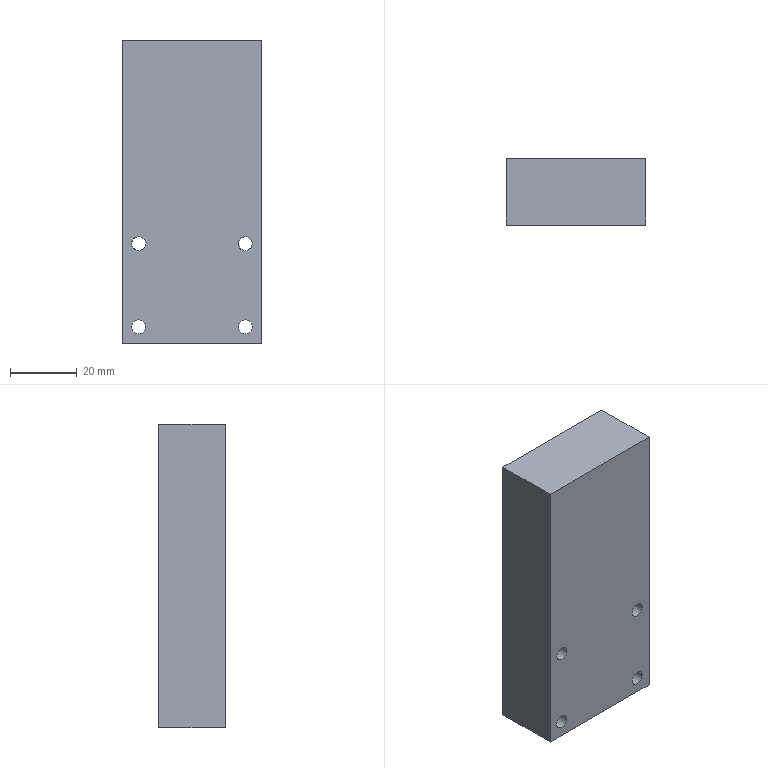Part | NX | features M5 螺纹孔1 2 | 1 solid | 10 faces | box 42 x 20 x 91 mm | volume 75332 mm3 | plane 6 | cylinder 4 | commonest cylinder face diameters 4.2 x4
STEP:
#1=CARTESIAN_POINT('',(16.,135.3,53.4));
#2=VERTEX_POINT('',#1);
#3=CARTESIAN_POINT('',(16.,135.3,55.5));
#4=DIRECTION('',(0.,-1.,0.));
#5=DIRECTION('',(0.,0.,-1.));
#6=AXIS2_PLACEMENT_3D('',#3,#4,#5);
#7=CIRCLE('',#6,2.1);
#8=EDGE_CURVE('',#2,#2,#7,.T.);
#9=ORIENTED_EDGE('',*,*,#8,.T.);
#10=EDGE_LOOP('',(#9));
#11=FACE_BOUND('',#10,.T.);
#12=CARTESIAN_POINT('',(16.,155.3,53.4));
#13=VERTEX_POINT('',#12);
#14=CARTESIAN_POINT('',(16.,155.3,55.5));
#15=DIRECTION('',(0.,-1.,0.));
#16=DIRECTION('',(0.,0.,-1.));
#17=AXIS2_PLACEMENT_3D('',#14,#15,#16);
#18=CIRCLE('',#17,2.1);
#19=EDGE_CURVE('',#13,#13,#18,.T.);
#20=ORIENTED_EDGE('',*,*,#19,.F.);
#21=EDGE_LOOP('',(#20));
#22=FACE_BOUND('',#21,.T.);
#23=CARTESIAN_POINT('',(16.,135.3,55.5));
#24=DIRECTION('',(0.,-1.,0.));
#25=DIRECTION('',(1.,0.,-0.000000009));
#26=AXIS2_PLACEMENT_3D('',#23,#24,#25);
#27=CYLINDRICAL_SURFACE('',#26,2.1);
#28=ADVANCED_FACE('',(#11,#22),#27,.F.);
#29=CARTESIAN_POINT('',(-16.,135.3,53.4));
#30=VERTEX_POINT('',#29);
#31=CARTESIAN_POINT('',(-16.,135.3,55.5));
#32=DIRECTION('',(0.,-1.,0.));
#33=DIRECTION('',(0.,0.,-1.));
#34=AXIS2_PLACEMENT_3D('',#31,#32,#33);
#35=CIRCLE('',#34,2.1);
#36=EDGE_CURVE('',#30,#30,#35,.T.);
#37=ORIENTED_EDGE('',*,*,#36,.T.);
#38=EDGE_LOOP('',(#37));
#39=FACE_BOUND('',#38,.T.);
#40=CARTESIAN_POINT('',(-16.,155.3,53.4));
#41=VERTEX_POINT('',#40);
#42=CARTESIAN_POINT('',(-16.,155.3,55.5));
#43=DIRECTION('',(0.,-1.,0.));
#44=DIRECTION('',(0.,0.,-1.));
#45=AXIS2_PLACEMENT_3D('',#42,#43,#44);
#46=CIRCLE('',#45,2.1);
#47=EDGE_CURVE('',#41,#41,#46,.T.);
#48=ORIENTED_EDGE('',*,*,#47,.F.);
#49=EDGE_LOOP('',(#48));
#50=FACE_BOUND('',#49,.T.);
#51=CARTESIAN_POINT('',(-16.,135.3,55.5));
#52=DIRECTION('',(0.,-1.,0.));
#53=DIRECTION('',(1.,0.,-0.000000009));
#54=AXIS2_PLACEMENT_3D('',#51,#52,#53);
#55=CYLINDRICAL_SURFACE('',#54,2.1);
#56=ADVANCED_FACE('',(#39,#50),#55,.F.);
#57=CARTESIAN_POINT('',(-21.,155.3,141.5));
#58=VERTEX_POINT('',#57);
#59=CARTESIAN_POINT('',(-21.,155.3,50.5));
#60=VERTEX_POINT('',#59);
#61=CARTESIAN_POINT('',(-21.,155.3,85.5));
#62=DIRECTION('',(-0.000000009,0.,-1.));
#63=VECTOR('',#62,1000.);
#64=LINE('',#61,#63);
#65=EDGE_CURVE('',#58,#60,#64,.T.);
#66=ORIENTED_EDGE('',*,*,#65,.T.);
#67=CARTESIAN_POINT('',(-21.,135.3,50.5));
#68=VERTEX_POINT('',#67);
#69=CARTESIAN_POINT('',(-21.,135.3,50.5));
#70=DIRECTION('',(0.,-1.,0.));
#71=VECTOR('',#70,1000.);
#72=LINE('',#69,#71);
#73=EDGE_CURVE('',#60,#68,#72,.T.);
#74=ORIENTED_EDGE('',*,*,#73,.T.);
#75=CARTESIAN_POINT('',(-21.,135.3,141.5));
#76=VERTEX_POINT('',#75);
#77=CARTESIAN_POINT('',(-21.,135.3,85.5));
#78=DIRECTION('',(0.000000009,0.,1.));
#79=VECTOR('',#78,1000.);
#80=LINE('',#77,#79);
#81=EDGE_CURVE('',#76,#68,#80,.F.);
#82=ORIENTED_EDGE('',*,*,#81,.F.);
#83=CARTESIAN_POINT('',(-21.,160.6,141.5));
#84=DIRECTION('',(0.,-1.,0.));
#85=VECTOR('',#84,1000.);
#86=LINE('',#83,#85);
#87=EDGE_CURVE('',#58,#76,#86,.T.);
#88=ORIENTED_EDGE('',*,*,#87,.F.);
#89=EDGE_LOOP('',(#66,#74,#82,#88));
#90=FACE_BOUND('',#89,.T.);
#91=CARTESIAN_POINT('',(-21.,135.3,85.5));
#92=DIRECTION('',(1.,0.,-0.000000009));
#93=DIRECTION('',(0.000000009,0.,1.));
#94=AXIS2_PLACEMENT_3D('',#91,#92,#93);
#95=PLANE('',#94);
#96=ADVANCED_FACE('',(#90),#95,.F.);
#97=CARTESIAN_POINT('',(21.,155.3,50.5));
#98=VERTEX_POINT('',#97);
#99=CARTESIAN_POINT('',(-25.,155.3,50.5));
#100=DIRECTION('',(1.,0.,-0.000000009));
#101=VECTOR('',#100,1000.);
#102=LINE('',#99,#101);
#103=EDGE_CURVE('',#60,#98,#102,.T.);
#104=ORIENTED_EDGE('',*,*,#103,.T.);
#105=CARTESIAN_POINT('',(21.,135.3,50.5));
#106=VERTEX_POINT('',#105);
#107=CARTESIAN_POINT('',(21.,89.3,50.5));
#108=DIRECTION('',(0.,-1.,0.));
#109=VECTOR('',#108,1000.);
#110=LINE('',#107,#109);
#111=EDGE_CURVE('',#98,#106,#110,.T.);
#112=ORIENTED_EDGE('',*,*,#111,.T.);
#113=CARTESIAN_POINT('',(-25.,135.3,50.5));
#114=DIRECTION('',(1.,0.,-0.000000009));
#115=VECTOR('',#114,1000.);
#116=LINE('',#113,#115);
#117=EDGE_CURVE('',#68,#106,#116,.T.);
#118=ORIENTED_EDGE('',*,*,#117,.F.);
#119=ORIENTED_EDGE('',*,*,#73,.F.);
#120=EDGE_LOOP('',(#104,#112,#118,#119));
#121=FACE_BOUND('',#120,.T.);
#122=CARTESIAN_POINT('',(-25.,89.3,50.5));
#123=DIRECTION('',(0.000000009,0.,1.));
#124=DIRECTION('',(0.,1.,0.));
#125=AXIS2_PLACEMENT_3D('',#122,#123,#124);
#126=PLANE('',#125);
#127=ADVANCED_FACE('',(#121),#126,.F.);
#128=CARTESIAN_POINT('',(21.,155.3,141.5));
#129=VERTEX_POINT('',#128);
#130=CARTESIAN_POINT('',(21.,155.3,85.5));
#131=DIRECTION('',(0.000000009,0.,1.));
#132=VECTOR('',#131,1000.);
#133=LINE('',#130,#132);
#134=EDGE_CURVE('',#98,#129,#133,.T.);
#135=ORIENTED_EDGE('',*,*,#134,.T.);
#136=CARTESIAN_POINT('',(21.,135.3,141.5));
#137=VERTEX_POINT('',#136);
#138=CARTESIAN_POINT('',(21.,135.3,141.5));
#139=DIRECTION('',(0.,-1.,0.));
#140=VECTOR('',#139,1000.);
#141=LINE('',#138,#140);
#142=EDGE_CURVE('',#129,#137,#141,.T.);
#143=ORIENTED_EDGE('',*,*,#142,.T.);
#144=CARTESIAN_POINT('',(21.,135.3,85.5));
#145=DIRECTION('',(-0.000000009,0.,-1.));
#146=VECTOR('',#145,1000.);
#147=LINE('',#144,#146);
#148=EDGE_CURVE('',#106,#137,#147,.F.);
#149=ORIENTED_EDGE('',*,*,#148,.F.);
#150=ORIENTED_EDGE('',*,*,#111,.F.);
#151=EDGE_LOOP('',(#135,#143,#149,#150));
#152=FACE_BOUND('',#151,.T.);
#153=CARTESIAN_POINT('',(21.,135.3,85.5));
#154=DIRECTION('',(-1.,0.,0.000000009));
#155=DIRECTION('',(-0.000000009,0.,-1.));
#156=AXIS2_PLACEMENT_3D('',#153,#154,#155);
#157=PLANE('',#156);
#158=ADVANCED_FACE('',(#152),#157,.F.);
#159=CARTESIAN_POINT('',(58.,155.3,141.5));
#160=DIRECTION('',(-1.,0.,0.000000019));
#161=VECTOR('',#160,1000.);
#162=LINE('',#159,#161);
#163=EDGE_CURVE('',#129,#58,#162,.T.);
#164=ORIENTED_EDGE('',*,*,#163,.T.);
#165=ORIENTED_EDGE('',*,*,#87,.T.);
#166=CARTESIAN_POINT('',(58.,135.3,141.5));
#167=DIRECTION('',(-1.,0.,0.000000019));
#168=VECTOR('',#167,1000.);
#169=LINE('',#166,#168);
#170=EDGE_CURVE('',#137,#76,#169,.T.);
#171=ORIENTED_EDGE('',*,*,#170,.F.);
#172=ORIENTED_EDGE('',*,*,#142,.F.);
#173=EDGE_LOOP('',(#164,#165,#171,#172));
#174=FACE_BOUND('',#173,.T.);
#175=CARTESIAN_POINT('',(58.,160.6,141.5));
#176=DIRECTION('',(-0.000000019,0.,-1.));
#177=DIRECTION('',(1.,0.,-0.000000019));
#178=AXIS2_PLACEMENT_3D('',#175,#176,#177);
#179=PLANE('',#178);
#180=ADVANCED_FACE('',(#174),#179,.F.);
#181=CARTESIAN_POINT('',(13.9,135.3,80.5));
#182=VERTEX_POINT('',#181);
#183=CARTESIAN_POINT('',(16.,135.3,80.5));
#184=DIRECTION('',(0.,1.,0.));
#185=DIRECTION('',(-1.,0.,0.000000009));
#186=AXIS2_PLACEMENT_3D('',#183,#184,#185);
#187=CIRCLE('',#186,2.1);
#188=EDGE_CURVE('',#182,#182,#187,.F.);
#189=ORIENTED_EDGE('',*,*,#188,.T.);
#190=EDGE_LOOP('',(#189));
#191=FACE_BOUND('',#190,.T.);
#192=CARTESIAN_POINT('',(16.,155.3,78.4));
#193=VERTEX_POINT('',#192);
#194=CARTESIAN_POINT('',(16.,155.3,80.5));
#195=DIRECTION('',(0.,-1.,0.));
#196=DIRECTION('',(0.,0.,-1.));
#197=AXIS2_PLACEMENT_3D('',#194,#195,#196);
#198=CIRCLE('',#197,2.1);
#199=EDGE_CURVE('',#193,#193,#198,.T.);
#200=ORIENTED_EDGE('',*,*,#199,.F.);
#201=EDGE_LOOP('',(#200));
#202=FACE_BOUND('',#201,.T.);
#203=CARTESIAN_POINT('',(16.,135.3,80.5));
#204=DIRECTION('',(0.,-1.,0.));
#205=DIRECTION('',(1.,0.,-0.000000009));
#206=AXIS2_PLACEMENT_3D('',#203,#204,#205);
#207=CYLINDRICAL_SURFACE('',#206,2.1);
#208=ADVANCED_FACE('',(#191,#202),#207,.F.);
#209=CARTESIAN_POINT('',(-18.1,135.3,80.5));
#210=VERTEX_POINT('',#209);
#211=CARTESIAN_POINT('',(-16.,135.3,80.5));
#212=DIRECTION('',(0.,1.,0.));
#213=DIRECTION('',(-1.,0.,0.000000009));
#214=AXIS2_PLACEMENT_3D('',#211,#212,#213);
#215=CIRCLE('',#214,2.1);
#216=EDGE_CURVE('',#210,#210,#215,.F.);
#217=ORIENTED_EDGE('',*,*,#216,.T.);
#218=EDGE_LOOP('',(#217));
#219=FACE_BOUND('',#218,.T.);
#220=CARTESIAN_POINT('',(-16.,155.3,78.4));
#221=VERTEX_POINT('',#220);
#222=CARTESIAN_POINT('',(-16.,155.3,80.5));
#223=DIRECTION('',(0.,-1.,0.));
#224=DIRECTION('',(0.,0.,-1.));
#225=AXIS2_PLACEMENT_3D('',#222,#223,#224);
#226=CIRCLE('',#225,2.1);
#227=EDGE_CURVE('',#221,#221,#226,.T.);
#228=ORIENTED_EDGE('',*,*,#227,.F.);
#229=EDGE_LOOP('',(#228));
#230=FACE_BOUND('',#229,.T.);
#231=CARTESIAN_POINT('',(-16.,135.3,80.5));
#232=DIRECTION('',(0.,-1.,0.));
#233=DIRECTION('',(1.,0.,-0.000000009));
#234=AXIS2_PLACEMENT_3D('',#231,#232,#233);
#235=CYLINDRICAL_SURFACE('',#234,2.1);
#236=ADVANCED_FACE('',(#219,#230),#235,.F.);
#237=ORIENTED_EDGE('',*,*,#19,.T.);
#238=EDGE_LOOP('',(#237));
#239=FACE_BOUND('',#238,.T.);
#240=ORIENTED_EDGE('',*,*,#47,.T.);
#241=EDGE_LOOP('',(#240));
#242=FACE_BOUND('',#241,.T.);
#243=ORIENTED_EDGE('',*,*,#227,.T.);
#244=EDGE_LOOP('',(#243));
#245=FACE_BOUND('',#244,.T.);
#246=ORIENTED_EDGE('',*,*,#199,.T.);
#247=EDGE_LOOP('',(#246));
#248=FACE_BOUND('',#247,.T.);
#249=ORIENTED_EDGE('',*,*,#163,.F.);
#250=ORIENTED_EDGE('',*,*,#134,.F.);
#251=ORIENTED_EDGE('',*,*,#103,.F.);
#252=ORIENTED_EDGE('',*,*,#65,.F.);
#253=EDGE_LOOP('',(#249,#250,#251,#252));
#254=FACE_BOUND('',#253,.T.);
#255=CARTESIAN_POINT('',(-0.000001581,155.3,70.5));
#256=DIRECTION('',(0.,-1.,0.));
#257=DIRECTION('',(1.,0.,-0.000000009));
#258=AXIS2_PLACEMENT_3D('',#255,#256,#257);
#259=PLANE('',#258);
#260=ADVANCED_FACE('',(#239,#242,#245,#248,#254),#259,.F.);
#261=ORIENTED_EDGE('',*,*,#8,.F.);
#262=EDGE_LOOP('',(#261));
#263=FACE_BOUND('',#262,.T.);
#264=ORIENTED_EDGE('',*,*,#36,.F.);
#265=EDGE_LOOP('',(#264));
#266=FACE_BOUND('',#265,.T.);
#267=ORIENTED_EDGE('',*,*,#148,.T.);
#268=ORIENTED_EDGE('',*,*,#170,.T.);
#269=ORIENTED_EDGE('',*,*,#81,.T.);
#270=ORIENTED_EDGE('',*,*,#117,.T.);
#271=EDGE_LOOP('',(#267,#268,#269,#270));
#272=FACE_BOUND('',#271,.T.);
#273=ORIENTED_EDGE('',*,*,#216,.F.);
#274=EDGE_LOOP('',(#273));
#275=FACE_BOUND('',#274,.T.);
#276=ORIENTED_EDGE('',*,*,#188,.F.);
#277=EDGE_LOOP('',(#276));
#278=FACE_BOUND('',#277,.T.);
#279=CARTESIAN_POINT('',(-0.000001581,135.3,70.5));
#280=DIRECTION('',(0.,-1.,0.));
#281=DIRECTION('',(1.,0.,-0.000000009));
#282=AXIS2_PLACEMENT_3D('',#279,#280,#281);
#283=PLANE('',#282);
#284=ADVANCED_FACE('',(#263,#266,#272,#275,#278),#283,.T.);
#285=CLOSED_SHELL('',(#28,#56,#96,#127,#158,#180,#208,#236,#260,#284));
#286=MANIFOLD_SOLID_BREP('',#285);
#287=(LENGTH_UNIT()NAMED_UNIT(*)SI_UNIT(.MILLI.,.METRE.));
#288=UNCERTAINTY_MEASURE_WITH_UNIT(LENGTH_MEASURE(0.00001),#287,'','');
#289=(NAMED_UNIT(*)PLANE_ANGLE_UNIT()SI_UNIT($,.RADIAN.));
#290=(NAMED_UNIT(*)SI_UNIT($,.STERADIAN.)SOLID_ANGLE_UNIT());
#291=(GEOMETRIC_REPRESENTATION_CONTEXT(3)GLOBAL_UNCERTAINTY_ASSIGNED_CONTEXT((#288))GLOBAL_UNIT_ASSIGNED_CONTEXT((#287,#289,#290))REPRESENTATION_CONTEXT('',''));
#292=ADVANCED_BREP_SHAPE_REPRESENTATION('',(#286),#291);